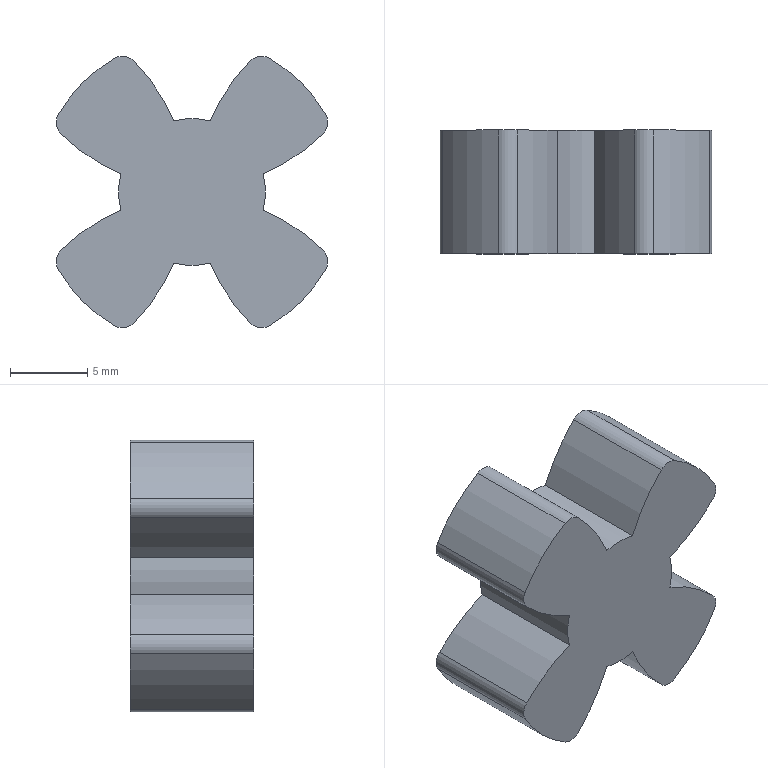Part | NX | features SPACER_5003_022_GCJC20-BL-6-8 2 | 1 solid | 26 faces | box 17.588 x 8 x 17.588 mm | volume 1623 mm3 | cylinder 24 | plane 2 | commonest cylinder face diameters 2 x8 24 x8 9.5 x4 20 x4
STEP:
#1=CARTESIAN_POINT('',(-225.435,-577.6,-105.5));
#2=VERTEX_POINT('',#1);
#3=CARTESIAN_POINT('',(-225.435,-569.6,-105.5));
#4=VERTEX_POINT('',#3);
#5=CARTESIAN_POINT('',(-225.435,-577.6,-105.5));
#6=DIRECTION('',(0.,1.,0.));
#7=VECTOR('',#6,1000.);
#8=LINE('',#5,#7);
#9=EDGE_CURVE('',#2,#4,#8,.T.);
#10=ORIENTED_EDGE('',*,*,#9,.F.);
#11=CARTESIAN_POINT('',(-221.775,-577.6,-101.84));
#12=VERTEX_POINT('',#11);
#13=CARTESIAN_POINT('',(-216.775,-577.6,-110.5));
#14=DIRECTION('',(0.,-1.,0.));
#15=DIRECTION('',(1.,0.,0.));
#16=AXIS2_PLACEMENT_3D('',#13,#14,#15);
#17=CIRCLE('',#16,10.);
#18=EDGE_CURVE('',#12,#2,#17,.T.);
#19=ORIENTED_EDGE('',*,*,#18,.F.);
#20=CARTESIAN_POINT('',(-221.775,-569.6,-101.84));
#21=VERTEX_POINT('',#20);
#22=CARTESIAN_POINT('',(-221.775,-577.6,-101.84));
#23=DIRECTION('',(0.,1.,0.));
#24=VECTOR('',#23,1000.);
#25=LINE('',#22,#24);
#26=EDGE_CURVE('',#12,#21,#25,.T.);
#27=ORIENTED_EDGE('',*,*,#26,.T.);
#28=CARTESIAN_POINT('',(-216.775,-569.6,-110.5));
#29=DIRECTION('',(0.,-1.,0.));
#30=DIRECTION('',(1.,0.,0.));
#31=AXIS2_PLACEMENT_3D('',#28,#29,#30);
#32=CIRCLE('',#31,10.);
#33=EDGE_CURVE('',#21,#4,#32,.T.);
#34=ORIENTED_EDGE('',*,*,#33,.T.);
#35=EDGE_LOOP('',(#10,#19,#27,#34));
#36=FACE_BOUND('',#35,.T.);
#37=CARTESIAN_POINT('',(-216.775,-577.6,-110.5));
#38=DIRECTION('',(0.,1.,0.));
#39=DIRECTION('',(-1.,0.,0.));
#40=AXIS2_PLACEMENT_3D('',#37,#38,#39);
#41=CYLINDRICAL_SURFACE('',#40,10.);
#42=ADVANCED_FACE('',(#36),#41,.T.);
#43=ORIENTED_EDGE('',*,*,#18,.T.);
#44=CARTESIAN_POINT('',(-225.278,-577.6,-106.706));
#45=VERTEX_POINT('',#44);
#46=CARTESIAN_POINT('',(-224.569,-577.6,-106.));
#47=DIRECTION('',(0.,1.,0.));
#48=DIRECTION('',(1.,0.,0.));
#49=AXIS2_PLACEMENT_3D('',#46,#47,#48);
#50=CIRCLE('',#49,1.);
#51=EDGE_CURVE('',#45,#2,#50,.T.);
#52=ORIENTED_EDGE('',*,*,#51,.F.);
#53=CARTESIAN_POINT('',(-221.376,-577.6,-109.321));
#54=VERTEX_POINT('',#53);
#55=CARTESIAN_POINT('',(-216.775,-577.6,-98.238));
#56=DIRECTION('',(0.,1.,0.));
#57=DIRECTION('',(1.,0.,0.));
#58=AXIS2_PLACEMENT_3D('',#55,#56,#57);
#59=CIRCLE('',#58,12.);
#60=EDGE_CURVE('',#54,#45,#59,.T.);
#61=ORIENTED_EDGE('',*,*,#60,.F.);
#62=CARTESIAN_POINT('',(-221.376,-577.6,-111.679));
#63=VERTEX_POINT('',#62);
#64=CARTESIAN_POINT('',(-216.775,-577.6,-110.5));
#65=DIRECTION('',(0.,1.,0.));
#66=DIRECTION('',(1.,0.,0.));
#67=AXIS2_PLACEMENT_3D('',#64,#65,#66);
#68=CIRCLE('',#67,4.75);
#69=EDGE_CURVE('',#63,#54,#68,.T.);
#70=ORIENTED_EDGE('',*,*,#69,.F.);
#71=CARTESIAN_POINT('',(-225.278,-577.6,-114.294));
#72=VERTEX_POINT('',#71);
#73=CARTESIAN_POINT('',(-216.775,-577.6,-122.762));
#74=DIRECTION('',(0.,1.,0.));
#75=DIRECTION('',(1.,0.,0.));
#76=AXIS2_PLACEMENT_3D('',#73,#74,#75);
#77=CIRCLE('',#76,12.);
#78=EDGE_CURVE('',#72,#63,#77,.T.);
#79=ORIENTED_EDGE('',*,*,#78,.F.);
#80=CARTESIAN_POINT('',(-225.435,-577.6,-115.5));
#81=VERTEX_POINT('',#80);
#82=CARTESIAN_POINT('',(-224.569,-577.6,-115.));
#83=DIRECTION('',(0.,1.,0.));
#84=DIRECTION('',(1.,0.,0.));
#85=AXIS2_PLACEMENT_3D('',#82,#83,#84);
#86=CIRCLE('',#85,1.);
#87=EDGE_CURVE('',#81,#72,#86,.T.);
#88=ORIENTED_EDGE('',*,*,#87,.F.);
#89=CARTESIAN_POINT('',(-221.775,-577.6,-119.16));
#90=VERTEX_POINT('',#89);
#91=CARTESIAN_POINT('',(-216.775,-577.6,-110.5));
#92=DIRECTION('',(0.,-1.,0.));
#93=DIRECTION('',(1.,0.,0.));
#94=AXIS2_PLACEMENT_3D('',#91,#92,#93);
#95=CIRCLE('',#94,10.);
#96=EDGE_CURVE('',#81,#90,#95,.T.);
#97=ORIENTED_EDGE('',*,*,#96,.T.);
#98=CARTESIAN_POINT('',(-220.569,-577.6,-119.003));
#99=VERTEX_POINT('',#98);
#100=CARTESIAN_POINT('',(-221.275,-577.6,-118.294));
#101=DIRECTION('',(0.,1.,0.));
#102=DIRECTION('',(1.,0.,0.));
#103=AXIS2_PLACEMENT_3D('',#100,#101,#102);
#104=CIRCLE('',#103,1.);
#105=EDGE_CURVE('',#99,#90,#104,.T.);
#106=ORIENTED_EDGE('',*,*,#105,.F.);
#107=CARTESIAN_POINT('',(-217.954,-577.6,-115.101));
#108=VERTEX_POINT('',#107);
#109=CARTESIAN_POINT('',(-229.037,-577.6,-110.5));
#110=DIRECTION('',(0.,1.,0.));
#111=DIRECTION('',(1.,0.,0.));
#112=AXIS2_PLACEMENT_3D('',#109,#110,#111);
#113=CIRCLE('',#112,12.);
#114=EDGE_CURVE('',#108,#99,#113,.T.);
#115=ORIENTED_EDGE('',*,*,#114,.F.);
#116=CARTESIAN_POINT('',(-215.596,-577.6,-115.101));
#117=VERTEX_POINT('',#116);
#118=CARTESIAN_POINT('',(-216.775,-577.6,-110.5));
#119=DIRECTION('',(0.,1.,0.));
#120=DIRECTION('',(1.,0.,0.));
#121=AXIS2_PLACEMENT_3D('',#118,#119,#120);
#122=CIRCLE('',#121,4.75);
#123=EDGE_CURVE('',#117,#108,#122,.T.);
#124=ORIENTED_EDGE('',*,*,#123,.F.);
#125=CARTESIAN_POINT('',(-212.981,-577.6,-119.003));
#126=VERTEX_POINT('',#125);
#127=CARTESIAN_POINT('',(-204.513,-577.6,-110.5));
#128=DIRECTION('',(0.,1.,0.));
#129=DIRECTION('',(1.,0.,0.));
#130=AXIS2_PLACEMENT_3D('',#127,#128,#129);
#131=CIRCLE('',#130,12.);
#132=EDGE_CURVE('',#126,#117,#131,.T.);
#133=ORIENTED_EDGE('',*,*,#132,.F.);
#134=CARTESIAN_POINT('',(-211.775,-577.6,-119.16));
#135=VERTEX_POINT('',#134);
#136=CARTESIAN_POINT('',(-212.275,-577.6,-118.294));
#137=DIRECTION('',(0.,1.,0.));
#138=DIRECTION('',(1.,0.,0.));
#139=AXIS2_PLACEMENT_3D('',#136,#137,#138);
#140=CIRCLE('',#139,1.);
#141=EDGE_CURVE('',#135,#126,#140,.T.);
#142=ORIENTED_EDGE('',*,*,#141,.F.);
#143=CARTESIAN_POINT('',(-208.115,-577.6,-115.5));
#144=VERTEX_POINT('',#143);
#145=CARTESIAN_POINT('',(-216.775,-577.6,-110.5));
#146=DIRECTION('',(0.,-1.,0.));
#147=DIRECTION('',(1.,0.,0.));
#148=AXIS2_PLACEMENT_3D('',#145,#146,#147);
#149=CIRCLE('',#148,10.);
#150=EDGE_CURVE('',#135,#144,#149,.T.);
#151=ORIENTED_EDGE('',*,*,#150,.T.);
#152=CARTESIAN_POINT('',(-208.272,-577.6,-114.294));
#153=VERTEX_POINT('',#152);
#154=CARTESIAN_POINT('',(-208.981,-577.6,-115.));
#155=DIRECTION('',(0.,1.,0.));
#156=DIRECTION('',(1.,0.,0.));
#157=AXIS2_PLACEMENT_3D('',#154,#155,#156);
#158=CIRCLE('',#157,1.);
#159=EDGE_CURVE('',#153,#144,#158,.T.);
#160=ORIENTED_EDGE('',*,*,#159,.F.);
#161=CARTESIAN_POINT('',(-212.174,-577.6,-111.679));
#162=VERTEX_POINT('',#161);
#163=CARTESIAN_POINT('',(-216.775,-577.6,-122.762));
#164=DIRECTION('',(0.,1.,0.));
#165=DIRECTION('',(1.,0.,0.));
#166=AXIS2_PLACEMENT_3D('',#163,#164,#165);
#167=CIRCLE('',#166,12.);
#168=EDGE_CURVE('',#162,#153,#167,.T.);
#169=ORIENTED_EDGE('',*,*,#168,.F.);
#170=CARTESIAN_POINT('',(-212.174,-577.6,-109.321));
#171=VERTEX_POINT('',#170);
#172=CARTESIAN_POINT('',(-216.775,-577.6,-110.5));
#173=DIRECTION('',(0.,1.,0.));
#174=DIRECTION('',(1.,0.,0.));
#175=AXIS2_PLACEMENT_3D('',#172,#173,#174);
#176=CIRCLE('',#175,4.75);
#177=EDGE_CURVE('',#171,#162,#176,.T.);
#178=ORIENTED_EDGE('',*,*,#177,.F.);
#179=CARTESIAN_POINT('',(-208.272,-577.6,-106.706));
#180=VERTEX_POINT('',#179);
#181=CARTESIAN_POINT('',(-216.775,-577.6,-98.238));
#182=DIRECTION('',(0.,1.,0.));
#183=DIRECTION('',(1.,0.,0.));
#184=AXIS2_PLACEMENT_3D('',#181,#182,#183);
#185=CIRCLE('',#184,12.);
#186=EDGE_CURVE('',#180,#171,#185,.T.);
#187=ORIENTED_EDGE('',*,*,#186,.F.);
#188=CARTESIAN_POINT('',(-208.115,-577.6,-105.5));
#189=VERTEX_POINT('',#188);
#190=CARTESIAN_POINT('',(-208.981,-577.6,-106.));
#191=DIRECTION('',(0.,1.,0.));
#192=DIRECTION('',(1.,0.,0.));
#193=AXIS2_PLACEMENT_3D('',#190,#191,#192);
#194=CIRCLE('',#193,1.);
#195=EDGE_CURVE('',#189,#180,#194,.T.);
#196=ORIENTED_EDGE('',*,*,#195,.F.);
#197=CARTESIAN_POINT('',(-211.775,-577.6,-101.84));
#198=VERTEX_POINT('',#197);
#199=CARTESIAN_POINT('',(-216.775,-577.6,-110.5));
#200=DIRECTION('',(0.,-1.,0.));
#201=DIRECTION('',(1.,0.,0.));
#202=AXIS2_PLACEMENT_3D('',#199,#200,#201);
#203=CIRCLE('',#202,10.);
#204=EDGE_CURVE('',#189,#198,#203,.T.);
#205=ORIENTED_EDGE('',*,*,#204,.T.);
#206=CARTESIAN_POINT('',(-212.981,-577.6,-101.997));
#207=VERTEX_POINT('',#206);
#208=CARTESIAN_POINT('',(-212.275,-577.6,-102.706));
#209=DIRECTION('',(0.,1.,0.));
#210=DIRECTION('',(1.,0.,0.));
#211=AXIS2_PLACEMENT_3D('',#208,#209,#210);
#212=CIRCLE('',#211,1.);
#213=EDGE_CURVE('',#207,#198,#212,.T.);
#214=ORIENTED_EDGE('',*,*,#213,.F.);
#215=CARTESIAN_POINT('',(-215.596,-577.6,-105.899));
#216=VERTEX_POINT('',#215);
#217=CARTESIAN_POINT('',(-204.513,-577.6,-110.5));
#218=DIRECTION('',(0.,1.,0.));
#219=DIRECTION('',(1.,0.,0.));
#220=AXIS2_PLACEMENT_3D('',#217,#218,#219);
#221=CIRCLE('',#220,12.);
#222=EDGE_CURVE('',#216,#207,#221,.T.);
#223=ORIENTED_EDGE('',*,*,#222,.F.);
#224=CARTESIAN_POINT('',(-217.954,-577.6,-105.899));
#225=VERTEX_POINT('',#224);
#226=CARTESIAN_POINT('',(-216.775,-577.6,-110.5));
#227=DIRECTION('',(0.,1.,0.));
#228=DIRECTION('',(1.,0.,0.));
#229=AXIS2_PLACEMENT_3D('',#226,#227,#228);
#230=CIRCLE('',#229,4.75);
#231=EDGE_CURVE('',#225,#216,#230,.T.);
#232=ORIENTED_EDGE('',*,*,#231,.F.);
#233=CARTESIAN_POINT('',(-220.569,-577.6,-101.997));
#234=VERTEX_POINT('',#233);
#235=CARTESIAN_POINT('',(-229.037,-577.6,-110.5));
#236=DIRECTION('',(0.,1.,0.));
#237=DIRECTION('',(1.,0.,0.));
#238=AXIS2_PLACEMENT_3D('',#235,#236,#237);
#239=CIRCLE('',#238,12.);
#240=EDGE_CURVE('',#234,#225,#239,.T.);
#241=ORIENTED_EDGE('',*,*,#240,.F.);
#242=CARTESIAN_POINT('',(-221.275,-577.6,-102.706));
#243=DIRECTION('',(0.,1.,0.));
#244=DIRECTION('',(1.,0.,0.));
#245=AXIS2_PLACEMENT_3D('',#242,#243,#244);
#246=CIRCLE('',#245,1.);
#247=EDGE_CURVE('',#12,#234,#246,.T.);
#248=ORIENTED_EDGE('',*,*,#247,.F.);
#249=EDGE_LOOP('',(#43,#52,#61,#70,#79,#88,#97,#106,#115,#124,#133,#142,#151,#160,#169,#178,#187,#196,#205,#214,#223,#232,#241,#248));
#250=FACE_BOUND('',#249,.T.);
#251=CARTESIAN_POINT('',(-216.775,-577.6,-110.5));
#252=DIRECTION('',(0.,-1.,0.));
#253=DIRECTION('',(1.,0.,0.));
#254=AXIS2_PLACEMENT_3D('',#251,#252,#253);
#255=PLANE('',#254);
#256=ADVANCED_FACE('',(#250),#255,.T.);
#257=CARTESIAN_POINT('',(-225.278,-569.6,-106.706));
#258=VERTEX_POINT('',#257);
#259=CARTESIAN_POINT('',(-224.569,-569.6,-106.));
#260=DIRECTION('',(0.,1.,0.));
#261=DIRECTION('',(1.,0.,0.));
#262=AXIS2_PLACEMENT_3D('',#259,#260,#261);
#263=CIRCLE('',#262,1.);
#264=EDGE_CURVE('',#258,#4,#263,.T.);
#265=ORIENTED_EDGE('',*,*,#264,.T.);
#266=ORIENTED_EDGE('',*,*,#33,.F.);
#267=CARTESIAN_POINT('',(-220.569,-569.6,-101.997));
#268=VERTEX_POINT('',#267);
#269=CARTESIAN_POINT('',(-221.275,-569.6,-102.706));
#270=DIRECTION('',(0.,1.,0.));
#271=DIRECTION('',(1.,0.,0.));
#272=AXIS2_PLACEMENT_3D('',#269,#270,#271);
#273=CIRCLE('',#272,1.);
#274=EDGE_CURVE('',#21,#268,#273,.T.);
#275=ORIENTED_EDGE('',*,*,#274,.T.);
#276=CARTESIAN_POINT('',(-217.954,-569.6,-105.899));
#277=VERTEX_POINT('',#276);
#278=CARTESIAN_POINT('',(-229.037,-569.6,-110.5));
#279=DIRECTION('',(0.,1.,0.));
#280=DIRECTION('',(1.,0.,0.));
#281=AXIS2_PLACEMENT_3D('',#278,#279,#280);
#282=CIRCLE('',#281,12.);
#283=EDGE_CURVE('',#268,#277,#282,.T.);
#284=ORIENTED_EDGE('',*,*,#283,.T.);
#285=CARTESIAN_POINT('',(-215.596,-569.6,-105.899));
#286=VERTEX_POINT('',#285);
#287=CARTESIAN_POINT('',(-216.775,-569.6,-110.5));
#288=DIRECTION('',(0.,1.,0.));
#289=DIRECTION('',(1.,0.,0.));
#290=AXIS2_PLACEMENT_3D('',#287,#288,#289);
#291=CIRCLE('',#290,4.75);
#292=EDGE_CURVE('',#277,#286,#291,.T.);
#293=ORIENTED_EDGE('',*,*,#292,.T.);
#294=CARTESIAN_POINT('',(-212.981,-569.6,-101.997));
#295=VERTEX_POINT('',#294);
#296=CARTESIAN_POINT('',(-204.513,-569.6,-110.5));
#297=DIRECTION('',(0.,1.,0.));
#298=DIRECTION('',(1.,0.,0.));
#299=AXIS2_PLACEMENT_3D('',#296,#297,#298);
#300=CIRCLE('',#299,12.);
#301=EDGE_CURVE('',#286,#295,#300,.T.);
#302=ORIENTED_EDGE('',*,*,#301,.T.);
#303=CARTESIAN_POINT('',(-211.775,-569.6,-101.84));
#304=VERTEX_POINT('',#303);
#305=CARTESIAN_POINT('',(-212.275,-569.6,-102.706));
#306=DIRECTION('',(0.,1.,0.));
#307=DIRECTION('',(1.,0.,0.));
#308=AXIS2_PLACEMENT_3D('',#305,#306,#307);
#309=CIRCLE('',#308,1.);
#310=EDGE_CURVE('',#295,#304,#309,.T.);
#311=ORIENTED_EDGE('',*,*,#310,.T.);
#312=CARTESIAN_POINT('',(-208.115,-569.6,-105.5));
#313=VERTEX_POINT('',#312);
#314=CARTESIAN_POINT('',(-216.775,-569.6,-110.5));
#315=DIRECTION('',(0.,-1.,0.));
#316=DIRECTION('',(1.,0.,0.));
#317=AXIS2_PLACEMENT_3D('',#314,#315,#316);
#318=CIRCLE('',#317,10.);
#319=EDGE_CURVE('',#313,#304,#318,.T.);
#320=ORIENTED_EDGE('',*,*,#319,.F.);
#321=CARTESIAN_POINT('',(-208.272,-569.6,-106.706));
#322=VERTEX_POINT('',#321);
#323=CARTESIAN_POINT('',(-208.981,-569.6,-106.));
#324=DIRECTION('',(0.,1.,0.));
#325=DIRECTION('',(1.,0.,0.));
#326=AXIS2_PLACEMENT_3D('',#323,#324,#325);
#327=CIRCLE('',#326,1.);
#328=EDGE_CURVE('',#313,#322,#327,.T.);
#329=ORIENTED_EDGE('',*,*,#328,.T.);
#330=CARTESIAN_POINT('',(-212.174,-569.6,-109.321));
#331=VERTEX_POINT('',#330);
#332=CARTESIAN_POINT('',(-216.775,-569.6,-98.238));
#333=DIRECTION('',(0.,1.,0.));
#334=DIRECTION('',(1.,0.,0.));
#335=AXIS2_PLACEMENT_3D('',#332,#333,#334);
#336=CIRCLE('',#335,12.);
#337=EDGE_CURVE('',#322,#331,#336,.T.);
#338=ORIENTED_EDGE('',*,*,#337,.T.);
#339=CARTESIAN_POINT('',(-212.174,-569.6,-111.679));
#340=VERTEX_POINT('',#339);
#341=CARTESIAN_POINT('',(-216.775,-569.6,-110.5));
#342=DIRECTION('',(0.,1.,0.));
#343=DIRECTION('',(1.,0.,0.));
#344=AXIS2_PLACEMENT_3D('',#341,#342,#343);
#345=CIRCLE('',#344,4.75);
#346=EDGE_CURVE('',#331,#340,#345,.T.);
#347=ORIENTED_EDGE('',*,*,#346,.T.);
#348=CARTESIAN_POINT('',(-208.272,-569.6,-114.294));
#349=VERTEX_POINT('',#348);
#350=CARTESIAN_POINT('',(-216.775,-569.6,-122.762));
#351=DIRECTION('',(0.,1.,0.));
#352=DIRECTION('',(1.,0.,0.));
#353=AXIS2_PLACEMENT_3D('',#350,#351,#352);
#354=CIRCLE('',#353,12.);
#355=EDGE_CURVE('',#340,#349,#354,.T.);
#356=ORIENTED_EDGE('',*,*,#355,.T.);
#357=CARTESIAN_POINT('',(-208.115,-569.6,-115.5));
#358=VERTEX_POINT('',#357);
#359=CARTESIAN_POINT('',(-208.981,-569.6,-115.));
#360=DIRECTION('',(0.,1.,0.));
#361=DIRECTION('',(1.,0.,0.));
#362=AXIS2_PLACEMENT_3D('',#359,#360,#361);
#363=CIRCLE('',#362,1.);
#364=EDGE_CURVE('',#349,#358,#363,.T.);
#365=ORIENTED_EDGE('',*,*,#364,.T.);
#366=CARTESIAN_POINT('',(-211.775,-569.6,-119.16));
#367=VERTEX_POINT('',#366);
#368=CARTESIAN_POINT('',(-216.775,-569.6,-110.5));
#369=DIRECTION('',(0.,-1.,0.));
#370=DIRECTION('',(1.,0.,0.));
#371=AXIS2_PLACEMENT_3D('',#368,#369,#370);
#372=CIRCLE('',#371,10.);
#373=EDGE_CURVE('',#367,#358,#372,.T.);
#374=ORIENTED_EDGE('',*,*,#373,.F.);
#375=CARTESIAN_POINT('',(-212.981,-569.6,-119.003));
#376=VERTEX_POINT('',#375);
#377=CARTESIAN_POINT('',(-212.275,-569.6,-118.294));
#378=DIRECTION('',(0.,1.,0.));
#379=DIRECTION('',(1.,0.,0.));
#380=AXIS2_PLACEMENT_3D('',#377,#378,#379);
#381=CIRCLE('',#380,1.);
#382=EDGE_CURVE('',#367,#376,#381,.T.);
#383=ORIENTED_EDGE('',*,*,#382,.T.);
#384=CARTESIAN_POINT('',(-215.596,-569.6,-115.101));
#385=VERTEX_POINT('',#384);
#386=CARTESIAN_POINT('',(-204.513,-569.6,-110.5));
#387=DIRECTION('',(0.,1.,0.));
#388=DIRECTION('',(1.,0.,0.));
#389=AXIS2_PLACEMENT_3D('',#386,#387,#388);
#390=CIRCLE('',#389,12.);
#391=EDGE_CURVE('',#376,#385,#390,.T.);
#392=ORIENTED_EDGE('',*,*,#391,.T.);
#393=CARTESIAN_POINT('',(-217.954,-569.6,-115.101));
#394=VERTEX_POINT('',#393);
#395=CARTESIAN_POINT('',(-216.775,-569.6,-110.5));
#396=DIRECTION('',(0.,1.,0.));
#397=DIRECTION('',(1.,0.,0.));
#398=AXIS2_PLACEMENT_3D('',#395,#396,#397);
#399=CIRCLE('',#398,4.75);
#400=EDGE_CURVE('',#385,#394,#399,.T.);
#401=ORIENTED_EDGE('',*,*,#400,.T.);
#402=CARTESIAN_POINT('',(-220.569,-569.6,-119.003));
#403=VERTEX_POINT('',#402);
#404=CARTESIAN_POINT('',(-229.037,-569.6,-110.5));
#405=DIRECTION('',(0.,1.,0.));
#406=DIRECTION('',(1.,0.,0.));
#407=AXIS2_PLACEMENT_3D('',#404,#405,#406);
#408=CIRCLE('',#407,12.);
#409=EDGE_CURVE('',#394,#403,#408,.T.);
#410=ORIENTED_EDGE('',*,*,#409,.T.);
#411=CARTESIAN_POINT('',(-221.775,-569.6,-119.16));
#412=VERTEX_POINT('',#411);
#413=CARTESIAN_POINT('',(-221.275,-569.6,-118.294));
#414=DIRECTION('',(0.,1.,0.));
#415=DIRECTION('',(1.,0.,0.));
#416=AXIS2_PLACEMENT_3D('',#413,#414,#415);
#417=CIRCLE('',#416,1.);
#418=EDGE_CURVE('',#403,#412,#417,.T.);
#419=ORIENTED_EDGE('',*,*,#418,.T.);
#420=CARTESIAN_POINT('',(-225.435,-569.6,-115.5));
#421=VERTEX_POINT('',#420);
#422=CARTESIAN_POINT('',(-216.775,-569.6,-110.5));
#423=DIRECTION('',(0.,-1.,0.));
#424=DIRECTION('',(1.,0.,0.));
#425=AXIS2_PLACEMENT_3D('',#422,#423,#424);
#426=CIRCLE('',#425,10.);
#427=EDGE_CURVE('',#421,#412,#426,.T.);
#428=ORIENTED_EDGE('',*,*,#427,.F.);
#429=CARTESIAN_POINT('',(-225.278,-569.6,-114.294));
#430=VERTEX_POINT('',#429);
#431=CARTESIAN_POINT('',(-224.569,-569.6,-115.));
#432=DIRECTION('',(0.,1.,0.));
#433=DIRECTION('',(1.,0.,0.));
#434=AXIS2_PLACEMENT_3D('',#431,#432,#433);
#435=CIRCLE('',#434,1.);
#436=EDGE_CURVE('',#421,#430,#435,.T.);
#437=ORIENTED_EDGE('',*,*,#436,.T.);
#438=CARTESIAN_POINT('',(-221.376,-569.6,-111.679));
#439=VERTEX_POINT('',#438);
#440=CARTESIAN_POINT('',(-216.775,-569.6,-122.762));
#441=DIRECTION('',(0.,1.,0.));
#442=DIRECTION('',(1.,0.,0.));
#443=AXIS2_PLACEMENT_3D('',#440,#441,#442);
#444=CIRCLE('',#443,12.);
#445=EDGE_CURVE('',#430,#439,#444,.T.);
#446=ORIENTED_EDGE('',*,*,#445,.T.);
#447=CARTESIAN_POINT('',(-221.376,-569.6,-109.321));
#448=VERTEX_POINT('',#447);
#449=CARTESIAN_POINT('',(-216.775,-569.6,-110.5));
#450=DIRECTION('',(0.,1.,0.));
#451=DIRECTION('',(1.,0.,0.));
#452=AXIS2_PLACEMENT_3D('',#449,#450,#451);
#453=CIRCLE('',#452,4.75);
#454=EDGE_CURVE('',#439,#448,#453,.T.);
#455=ORIENTED_EDGE('',*,*,#454,.T.);
#456=CARTESIAN_POINT('',(-216.775,-569.6,-98.238));
#457=DIRECTION('',(0.,1.,0.));
#458=DIRECTION('',(1.,0.,0.));
#459=AXIS2_PLACEMENT_3D('',#456,#457,#458);
#460=CIRCLE('',#459,12.);
#461=EDGE_CURVE('',#448,#258,#460,.T.);
#462=ORIENTED_EDGE('',*,*,#461,.T.);
#463=EDGE_LOOP('',(#265,#266,#275,#284,#293,#302,#311,#320,#329,#338,#347,#356,#365,#374,#383,#392,#401,#410,#419,#428,#437,#446,#455,#462));
#464=FACE_BOUND('',#463,.T.);
#465=CARTESIAN_POINT('',(-216.775,-569.6,-110.5));
#466=DIRECTION('',(0.,-1.,0.));
#467=DIRECTION('',(1.,0.,0.));
#468=AXIS2_PLACEMENT_3D('',#465,#466,#467);
#469=PLANE('',#468);
#470=ADVANCED_FACE('',(#464),#469,.F.);
#471=ORIENTED_EDGE('',*,*,#96,.F.);
#472=CARTESIAN_POINT('',(-225.435,-577.6,-115.5));
#473=DIRECTION('',(0.,1.,0.));
#474=VECTOR('',#473,1000.);
#475=LINE('',#472,#474);
#476=EDGE_CURVE('',#81,#421,#475,.T.);
#477=ORIENTED_EDGE('',*,*,#476,.T.);
#478=ORIENTED_EDGE('',*,*,#427,.T.);
#479=CARTESIAN_POINT('',(-221.775,-577.6,-119.16));
#480=DIRECTION('',(0.,1.,0.));
#481=VECTOR('',#480,1000.);
#482=LINE('',#479,#481);
#483=EDGE_CURVE('',#90,#412,#482,.T.);
#484=ORIENTED_EDGE('',*,*,#483,.F.);
#485=EDGE_LOOP('',(#471,#477,#478,#484));
#486=FACE_BOUND('',#485,.T.);
#487=CARTESIAN_POINT('',(-216.775,-577.6,-110.5));
#488=DIRECTION('',(0.,1.,0.));
#489=DIRECTION('',(-1.,0.,0.));
#490=AXIS2_PLACEMENT_3D('',#487,#488,#489);
#491=CYLINDRICAL_SURFACE('',#490,10.);
#492=ADVANCED_FACE('',(#486),#491,.T.);
#493=ORIENTED_EDGE('',*,*,#150,.F.);
#494=CARTESIAN_POINT('',(-211.775,-577.6,-119.16));
#495=DIRECTION('',(0.,1.,0.));
#496=VECTOR('',#495,1000.);
#497=LINE('',#494,#496);
#498=EDGE_CURVE('',#135,#367,#497,.T.);
#499=ORIENTED_EDGE('',*,*,#498,.T.);
#500=ORIENTED_EDGE('',*,*,#373,.T.);
#501=CARTESIAN_POINT('',(-208.115,-577.6,-115.5));
#502=DIRECTION('',(0.,1.,0.));
#503=VECTOR('',#502,1000.);
#504=LINE('',#501,#503);
#505=EDGE_CURVE('',#144,#358,#504,.T.);
#506=ORIENTED_EDGE('',*,*,#505,.F.);
#507=EDGE_LOOP('',(#493,#499,#500,#506));
#508=FACE_BOUND('',#507,.T.);
#509=CARTESIAN_POINT('',(-216.775,-577.6,-110.5));
#510=DIRECTION('',(0.,1.,0.));
#511=DIRECTION('',(-1.,0.,0.));
#512=AXIS2_PLACEMENT_3D('',#509,#510,#511);
#513=CYLINDRICAL_SURFACE('',#512,10.);
#514=ADVANCED_FACE('',(#508),#513,.T.);
#515=ORIENTED_EDGE('',*,*,#204,.F.);
#516=CARTESIAN_POINT('',(-208.115,-577.6,-105.5));
#517=DIRECTION('',(0.,1.,0.));
#518=VECTOR('',#517,1000.);
#519=LINE('',#516,#518);
#520=EDGE_CURVE('',#189,#313,#519,.T.);
#521=ORIENTED_EDGE('',*,*,#520,.T.);
#522=ORIENTED_EDGE('',*,*,#319,.T.);
#523=CARTESIAN_POINT('',(-211.775,-577.6,-101.84));
#524=DIRECTION('',(0.,1.,0.));
#525=VECTOR('',#524,1000.);
#526=LINE('',#523,#525);
#527=EDGE_CURVE('',#198,#304,#526,.T.);
#528=ORIENTED_EDGE('',*,*,#527,.F.);
#529=EDGE_LOOP('',(#515,#521,#522,#528));
#530=FACE_BOUND('',#529,.T.);
#531=CARTESIAN_POINT('',(-216.775,-577.6,-110.5));
#532=DIRECTION('',(0.,1.,0.));
#533=DIRECTION('',(-1.,0.,0.));
#534=AXIS2_PLACEMENT_3D('',#531,#532,#533);
#535=CYLINDRICAL_SURFACE('',#534,10.);
#536=ADVANCED_FACE('',(#530),#535,.T.);
#537=ORIENTED_EDGE('',*,*,#310,.F.);
#538=CARTESIAN_POINT('',(-212.981,-577.6,-101.997));
#539=DIRECTION('',(0.,1.,0.));
#540=VECTOR('',#539,1000.);
#541=LINE('',#538,#540);
#542=EDGE_CURVE('',#207,#295,#541,.T.);
#543=ORIENTED_EDGE('',*,*,#542,.F.);
#544=ORIENTED_EDGE('',*,*,#213,.T.);
#545=ORIENTED_EDGE('',*,*,#527,.T.);
#546=EDGE_LOOP('',(#537,#543,#544,#545));
#547=FACE_BOUND('',#546,.T.);
#548=CARTESIAN_POINT('',(-212.275,-577.6,-102.706));
#549=DIRECTION('',(0.,1.,0.));
#550=DIRECTION('',(-1.,0.,0.));
#551=AXIS2_PLACEMENT_3D('',#548,#549,#550);
#552=CYLINDRICAL_SURFACE('',#551,1.);
#553=ADVANCED_FACE('',(#547),#552,.T.);
#554=ORIENTED_EDGE('',*,*,#274,.F.);
#555=ORIENTED_EDGE('',*,*,#26,.F.);
#556=ORIENTED_EDGE('',*,*,#247,.T.);
#557=CARTESIAN_POINT('',(-220.569,-577.6,-101.997));
#558=DIRECTION('',(0.,1.,0.));
#559=VECTOR('',#558,1000.);
#560=LINE('',#557,#559);
#561=EDGE_CURVE('',#234,#268,#560,.T.);
#562=ORIENTED_EDGE('',*,*,#561,.T.);
#563=EDGE_LOOP('',(#554,#555,#556,#562));
#564=FACE_BOUND('',#563,.T.);
#565=CARTESIAN_POINT('',(-221.275,-577.6,-102.706));
#566=DIRECTION('',(0.,1.,0.));
#567=DIRECTION('',(-1.,0.,0.));
#568=AXIS2_PLACEMENT_3D('',#565,#566,#567);
#569=CYLINDRICAL_SURFACE('',#568,1.);
#570=ADVANCED_FACE('',(#564),#569,.T.);
#571=ORIENTED_EDGE('',*,*,#283,.F.);
#572=ORIENTED_EDGE('',*,*,#561,.F.);
#573=ORIENTED_EDGE('',*,*,#240,.T.);
#574=CARTESIAN_POINT('',(-217.954,-577.6,-105.899));
#575=DIRECTION('',(0.,1.,0.));
#576=VECTOR('',#575,1000.);
#577=LINE('',#574,#576);
#578=EDGE_CURVE('',#225,#277,#577,.T.);
#579=ORIENTED_EDGE('',*,*,#578,.T.);
#580=EDGE_LOOP('',(#571,#572,#573,#579));
#581=FACE_BOUND('',#580,.T.);
#582=CARTESIAN_POINT('',(-229.037,-577.6,-110.5));
#583=DIRECTION('',(0.,1.,0.));
#584=DIRECTION('',(-1.,0.,0.));
#585=AXIS2_PLACEMENT_3D('',#582,#583,#584);
#586=CYLINDRICAL_SURFACE('',#585,12.);
#587=ADVANCED_FACE('',(#581),#586,.T.);
#588=ORIENTED_EDGE('',*,*,#292,.F.);
#589=ORIENTED_EDGE('',*,*,#578,.F.);
#590=ORIENTED_EDGE('',*,*,#231,.T.);
#591=CARTESIAN_POINT('',(-215.596,-577.6,-105.899));
#592=DIRECTION('',(0.,1.,0.));
#593=VECTOR('',#592,1000.);
#594=LINE('',#591,#593);
#595=EDGE_CURVE('',#216,#286,#594,.T.);
#596=ORIENTED_EDGE('',*,*,#595,.T.);
#597=EDGE_LOOP('',(#588,#589,#590,#596));
#598=FACE_BOUND('',#597,.T.);
#599=CARTESIAN_POINT('',(-216.775,-577.6,-110.5));
#600=DIRECTION('',(0.,1.,0.));
#601=DIRECTION('',(-1.,0.,0.));
#602=AXIS2_PLACEMENT_3D('',#599,#600,#601);
#603=CYLINDRICAL_SURFACE('',#602,4.75);
#604=ADVANCED_FACE('',(#598),#603,.T.);
#605=ORIENTED_EDGE('',*,*,#301,.F.);
#606=ORIENTED_EDGE('',*,*,#595,.F.);
#607=ORIENTED_EDGE('',*,*,#222,.T.);
#608=ORIENTED_EDGE('',*,*,#542,.T.);
#609=EDGE_LOOP('',(#605,#606,#607,#608));
#610=FACE_BOUND('',#609,.T.);
#611=CARTESIAN_POINT('',(-204.513,-577.6,-110.5));
#612=DIRECTION('',(0.,1.,0.));
#613=DIRECTION('',(-1.,0.,0.));
#614=AXIS2_PLACEMENT_3D('',#611,#612,#613);
#615=CYLINDRICAL_SURFACE('',#614,12.);
#616=ADVANCED_FACE('',(#610),#615,.T.);
#617=ORIENTED_EDGE('',*,*,#364,.F.);
#618=CARTESIAN_POINT('',(-208.272,-577.6,-114.294));
#619=DIRECTION('',(0.,1.,0.));
#620=VECTOR('',#619,1000.);
#621=LINE('',#618,#620);
#622=EDGE_CURVE('',#153,#349,#621,.T.);
#623=ORIENTED_EDGE('',*,*,#622,.F.);
#624=ORIENTED_EDGE('',*,*,#159,.T.);
#625=ORIENTED_EDGE('',*,*,#505,.T.);
#626=EDGE_LOOP('',(#617,#623,#624,#625));
#627=FACE_BOUND('',#626,.T.);
#628=CARTESIAN_POINT('',(-208.981,-577.6,-115.));
#629=DIRECTION('',(0.,1.,0.));
#630=DIRECTION('',(-1.,0.,0.));
#631=AXIS2_PLACEMENT_3D('',#628,#629,#630);
#632=CYLINDRICAL_SURFACE('',#631,1.);
#633=ADVANCED_FACE('',(#627),#632,.T.);
#634=ORIENTED_EDGE('',*,*,#328,.F.);
#635=ORIENTED_EDGE('',*,*,#520,.F.);
#636=ORIENTED_EDGE('',*,*,#195,.T.);
#637=CARTESIAN_POINT('',(-208.272,-577.6,-106.706));
#638=DIRECTION('',(0.,1.,0.));
#639=VECTOR('',#638,1000.);
#640=LINE('',#637,#639);
#641=EDGE_CURVE('',#180,#322,#640,.T.);
#642=ORIENTED_EDGE('',*,*,#641,.T.);
#643=EDGE_LOOP('',(#634,#635,#636,#642));
#644=FACE_BOUND('',#643,.T.);
#645=CARTESIAN_POINT('',(-208.981,-577.6,-106.));
#646=DIRECTION('',(0.,1.,0.));
#647=DIRECTION('',(-1.,0.,0.));
#648=AXIS2_PLACEMENT_3D('',#645,#646,#647);
#649=CYLINDRICAL_SURFACE('',#648,1.);
#650=ADVANCED_FACE('',(#644),#649,.T.);
#651=ORIENTED_EDGE('',*,*,#337,.F.);
#652=ORIENTED_EDGE('',*,*,#641,.F.);
#653=ORIENTED_EDGE('',*,*,#186,.T.);
#654=CARTESIAN_POINT('',(-212.174,-577.6,-109.321));
#655=DIRECTION('',(0.,1.,0.));
#656=VECTOR('',#655,1000.);
#657=LINE('',#654,#656);
#658=EDGE_CURVE('',#171,#331,#657,.T.);
#659=ORIENTED_EDGE('',*,*,#658,.T.);
#660=EDGE_LOOP('',(#651,#652,#653,#659));
#661=FACE_BOUND('',#660,.T.);
#662=CARTESIAN_POINT('',(-216.775,-577.6,-98.238));
#663=DIRECTION('',(0.,1.,0.));
#664=DIRECTION('',(-1.,0.,0.));
#665=AXIS2_PLACEMENT_3D('',#662,#663,#664);
#666=CYLINDRICAL_SURFACE('',#665,12.);
#667=ADVANCED_FACE('',(#661),#666,.T.);
#668=ORIENTED_EDGE('',*,*,#346,.F.);
#669=ORIENTED_EDGE('',*,*,#658,.F.);
#670=ORIENTED_EDGE('',*,*,#177,.T.);
#671=CARTESIAN_POINT('',(-212.174,-577.6,-111.679));
#672=DIRECTION('',(0.,1.,0.));
#673=VECTOR('',#672,1000.);
#674=LINE('',#671,#673);
#675=EDGE_CURVE('',#162,#340,#674,.T.);
#676=ORIENTED_EDGE('',*,*,#675,.T.);
#677=EDGE_LOOP('',(#668,#669,#670,#676));
#678=FACE_BOUND('',#677,.T.);
#679=CARTESIAN_POINT('',(-216.775,-577.6,-110.5));
#680=DIRECTION('',(0.,1.,0.));
#681=DIRECTION('',(-1.,0.,0.));
#682=AXIS2_PLACEMENT_3D('',#679,#680,#681);
#683=CYLINDRICAL_SURFACE('',#682,4.75);
#684=ADVANCED_FACE('',(#678),#683,.T.);
#685=ORIENTED_EDGE('',*,*,#355,.F.);
#686=ORIENTED_EDGE('',*,*,#675,.F.);
#687=ORIENTED_EDGE('',*,*,#168,.T.);
#688=ORIENTED_EDGE('',*,*,#622,.T.);
#689=EDGE_LOOP('',(#685,#686,#687,#688));
#690=FACE_BOUND('',#689,.T.);
#691=CARTESIAN_POINT('',(-216.775,-577.6,-122.762));
#692=DIRECTION('',(0.,1.,0.));
#693=DIRECTION('',(-1.,0.,0.));
#694=AXIS2_PLACEMENT_3D('',#691,#692,#693);
#695=CYLINDRICAL_SURFACE('',#694,12.);
#696=ADVANCED_FACE('',(#690),#695,.T.);
#697=ORIENTED_EDGE('',*,*,#418,.F.);
#698=CARTESIAN_POINT('',(-220.569,-577.6,-119.003));
#699=DIRECTION('',(0.,1.,0.));
#700=VECTOR('',#699,1000.);
#701=LINE('',#698,#700);
#702=EDGE_CURVE('',#99,#403,#701,.T.);
#703=ORIENTED_EDGE('',*,*,#702,.F.);
#704=ORIENTED_EDGE('',*,*,#105,.T.);
#705=ORIENTED_EDGE('',*,*,#483,.T.);
#706=EDGE_LOOP('',(#697,#703,#704,#705));
#707=FACE_BOUND('',#706,.T.);
#708=CARTESIAN_POINT('',(-221.275,-577.6,-118.294));
#709=DIRECTION('',(0.,1.,0.));
#710=DIRECTION('',(-1.,0.,0.));
#711=AXIS2_PLACEMENT_3D('',#708,#709,#710);
#712=CYLINDRICAL_SURFACE('',#711,1.);
#713=ADVANCED_FACE('',(#707),#712,.T.);
#714=ORIENTED_EDGE('',*,*,#382,.F.);
#715=ORIENTED_EDGE('',*,*,#498,.F.);
#716=ORIENTED_EDGE('',*,*,#141,.T.);
#717=CARTESIAN_POINT('',(-212.981,-577.6,-119.003));
#718=DIRECTION('',(0.,1.,0.));
#719=VECTOR('',#718,1000.);
#720=LINE('',#717,#719);
#721=EDGE_CURVE('',#126,#376,#720,.T.);
#722=ORIENTED_EDGE('',*,*,#721,.T.);
#723=EDGE_LOOP('',(#714,#715,#716,#722));
#724=FACE_BOUND('',#723,.T.);
#725=CARTESIAN_POINT('',(-212.275,-577.6,-118.294));
#726=DIRECTION('',(0.,1.,0.));
#727=DIRECTION('',(-1.,0.,0.));
#728=AXIS2_PLACEMENT_3D('',#725,#726,#727);
#729=CYLINDRICAL_SURFACE('',#728,1.);
#730=ADVANCED_FACE('',(#724),#729,.T.);
#731=ORIENTED_EDGE('',*,*,#391,.F.);
#732=ORIENTED_EDGE('',*,*,#721,.F.);
#733=ORIENTED_EDGE('',*,*,#132,.T.);
#734=CARTESIAN_POINT('',(-215.596,-577.6,-115.101));
#735=DIRECTION('',(0.,1.,0.));
#736=VECTOR('',#735,1000.);
#737=LINE('',#734,#736);
#738=EDGE_CURVE('',#117,#385,#737,.T.);
#739=ORIENTED_EDGE('',*,*,#738,.T.);
#740=EDGE_LOOP('',(#731,#732,#733,#739));
#741=FACE_BOUND('',#740,.T.);
#742=CARTESIAN_POINT('',(-204.513,-577.6,-110.5));
#743=DIRECTION('',(0.,1.,0.));
#744=DIRECTION('',(-1.,0.,0.));
#745=AXIS2_PLACEMENT_3D('',#742,#743,#744);
#746=CYLINDRICAL_SURFACE('',#745,12.);
#747=ADVANCED_FACE('',(#741),#746,.T.);
#748=ORIENTED_EDGE('',*,*,#400,.F.);
#749=ORIENTED_EDGE('',*,*,#738,.F.);
#750=ORIENTED_EDGE('',*,*,#123,.T.);
#751=CARTESIAN_POINT('',(-217.954,-577.6,-115.101));
#752=DIRECTION('',(0.,1.,0.));
#753=VECTOR('',#752,1000.);
#754=LINE('',#751,#753);
#755=EDGE_CURVE('',#108,#394,#754,.T.);
#756=ORIENTED_EDGE('',*,*,#755,.T.);
#757=EDGE_LOOP('',(#748,#749,#750,#756));
#758=FACE_BOUND('',#757,.T.);
#759=CARTESIAN_POINT('',(-216.775,-577.6,-110.5));
#760=DIRECTION('',(0.,1.,0.));
#761=DIRECTION('',(-1.,0.,0.));
#762=AXIS2_PLACEMENT_3D('',#759,#760,#761);
#763=CYLINDRICAL_SURFACE('',#762,4.75);
#764=ADVANCED_FACE('',(#758),#763,.T.);
#765=ORIENTED_EDGE('',*,*,#409,.F.);
#766=ORIENTED_EDGE('',*,*,#755,.F.);
#767=ORIENTED_EDGE('',*,*,#114,.T.);
#768=ORIENTED_EDGE('',*,*,#702,.T.);
#769=EDGE_LOOP('',(#765,#766,#767,#768));
#770=FACE_BOUND('',#769,.T.);
#771=CARTESIAN_POINT('',(-229.037,-577.6,-110.5));
#772=DIRECTION('',(0.,1.,0.));
#773=DIRECTION('',(-1.,0.,0.));
#774=AXIS2_PLACEMENT_3D('',#771,#772,#773);
#775=CYLINDRICAL_SURFACE('',#774,12.);
#776=ADVANCED_FACE('',(#770),#775,.T.);
#777=ORIENTED_EDGE('',*,*,#264,.F.);
#778=CARTESIAN_POINT('',(-225.278,-577.6,-106.706));
#779=DIRECTION('',(0.,1.,0.));
#780=VECTOR('',#779,1000.);
#781=LINE('',#778,#780);
#782=EDGE_CURVE('',#45,#258,#781,.T.);
#783=ORIENTED_EDGE('',*,*,#782,.F.);
#784=ORIENTED_EDGE('',*,*,#51,.T.);
#785=ORIENTED_EDGE('',*,*,#9,.T.);
#786=EDGE_LOOP('',(#777,#783,#784,#785));
#787=FACE_BOUND('',#786,.T.);
#788=CARTESIAN_POINT('',(-224.569,-577.6,-106.));
#789=DIRECTION('',(0.,1.,0.));
#790=DIRECTION('',(-1.,0.,0.));
#791=AXIS2_PLACEMENT_3D('',#788,#789,#790);
#792=CYLINDRICAL_SURFACE('',#791,1.);
#793=ADVANCED_FACE('',(#787),#792,.T.);
#794=ORIENTED_EDGE('',*,*,#436,.F.);
#795=ORIENTED_EDGE('',*,*,#476,.F.);
#796=ORIENTED_EDGE('',*,*,#87,.T.);
#797=CARTESIAN_POINT('',(-225.278,-577.6,-114.294));
#798=DIRECTION('',(0.,1.,0.));
#799=VECTOR('',#798,1000.);
#800=LINE('',#797,#799);
#801=EDGE_CURVE('',#72,#430,#800,.T.);
#802=ORIENTED_EDGE('',*,*,#801,.T.);
#803=EDGE_LOOP('',(#794,#795,#796,#802));
#804=FACE_BOUND('',#803,.T.);
#805=CARTESIAN_POINT('',(-224.569,-577.6,-115.));
#806=DIRECTION('',(0.,1.,0.));
#807=DIRECTION('',(-1.,0.,0.));
#808=AXIS2_PLACEMENT_3D('',#805,#806,#807);
#809=CYLINDRICAL_SURFACE('',#808,1.);
#810=ADVANCED_FACE('',(#804),#809,.T.);
#811=ORIENTED_EDGE('',*,*,#445,.F.);
#812=ORIENTED_EDGE('',*,*,#801,.F.);
#813=ORIENTED_EDGE('',*,*,#78,.T.);
#814=CARTESIAN_POINT('',(-221.376,-577.6,-111.679));
#815=DIRECTION('',(0.,1.,0.));
#816=VECTOR('',#815,1000.);
#817=LINE('',#814,#816);
#818=EDGE_CURVE('',#63,#439,#817,.T.);
#819=ORIENTED_EDGE('',*,*,#818,.T.);
#820=EDGE_LOOP('',(#811,#812,#813,#819));
#821=FACE_BOUND('',#820,.T.);
#822=CARTESIAN_POINT('',(-216.775,-577.6,-122.762));
#823=DIRECTION('',(0.,1.,0.));
#824=DIRECTION('',(-1.,0.,0.));
#825=AXIS2_PLACEMENT_3D('',#822,#823,#824);
#826=CYLINDRICAL_SURFACE('',#825,12.);
#827=ADVANCED_FACE('',(#821),#826,.T.);
#828=ORIENTED_EDGE('',*,*,#454,.F.);
#829=ORIENTED_EDGE('',*,*,#818,.F.);
#830=ORIENTED_EDGE('',*,*,#69,.T.);
#831=CARTESIAN_POINT('',(-221.376,-577.6,-109.321));
#832=DIRECTION('',(0.,1.,0.));
#833=VECTOR('',#832,1000.);
#834=LINE('',#831,#833);
#835=EDGE_CURVE('',#54,#448,#834,.T.);
#836=ORIENTED_EDGE('',*,*,#835,.T.);
#837=EDGE_LOOP('',(#828,#829,#830,#836));
#838=FACE_BOUND('',#837,.T.);
#839=CARTESIAN_POINT('',(-216.775,-577.6,-110.5));
#840=DIRECTION('',(0.,1.,0.));
#841=DIRECTION('',(-1.,0.,0.));
#842=AXIS2_PLACEMENT_3D('',#839,#840,#841);
#843=CYLINDRICAL_SURFACE('',#842,4.75);
#844=ADVANCED_FACE('',(#838),#843,.T.);
#845=ORIENTED_EDGE('',*,*,#461,.F.);
#846=ORIENTED_EDGE('',*,*,#835,.F.);
#847=ORIENTED_EDGE('',*,*,#60,.T.);
#848=ORIENTED_EDGE('',*,*,#782,.T.);
#849=EDGE_LOOP('',(#845,#846,#847,#848));
#850=FACE_BOUND('',#849,.T.);
#851=CARTESIAN_POINT('',(-216.775,-577.6,-98.238));
#852=DIRECTION('',(0.,1.,0.));
#853=DIRECTION('',(-1.,0.,0.));
#854=AXIS2_PLACEMENT_3D('',#851,#852,#853);
#855=CYLINDRICAL_SURFACE('',#854,12.);
#856=ADVANCED_FACE('',(#850),#855,.T.);
#857=CLOSED_SHELL('',(#42,#256,#470,#492,#514,#536,#553,#570,#587,#604,#616,#633,#650,#667,#684,#696,#713,#730,#747,#764,#776,#793,#810,#827,#844,#856));
#858=MANIFOLD_SOLID_BREP('',#857);
#859=(LENGTH_UNIT()NAMED_UNIT(*)SI_UNIT(.MILLI.,.METRE.));
#860=UNCERTAINTY_MEASURE_WITH_UNIT(LENGTH_MEASURE(0.00001),#859,'','');
#861=(NAMED_UNIT(*)PLANE_ANGLE_UNIT()SI_UNIT($,.RADIAN.));
#862=(NAMED_UNIT(*)SI_UNIT($,.STERADIAN.)SOLID_ANGLE_UNIT());
#863=(GEOMETRIC_REPRESENTATION_CONTEXT(3)GLOBAL_UNCERTAINTY_ASSIGNED_CONTEXT((#860))GLOBAL_UNIT_ASSIGNED_CONTEXT((#859,#861,#862))REPRESENTATION_CONTEXT('',''));
#864=ADVANCED_BREP_SHAPE_REPRESENTATION('',(#858),#863);